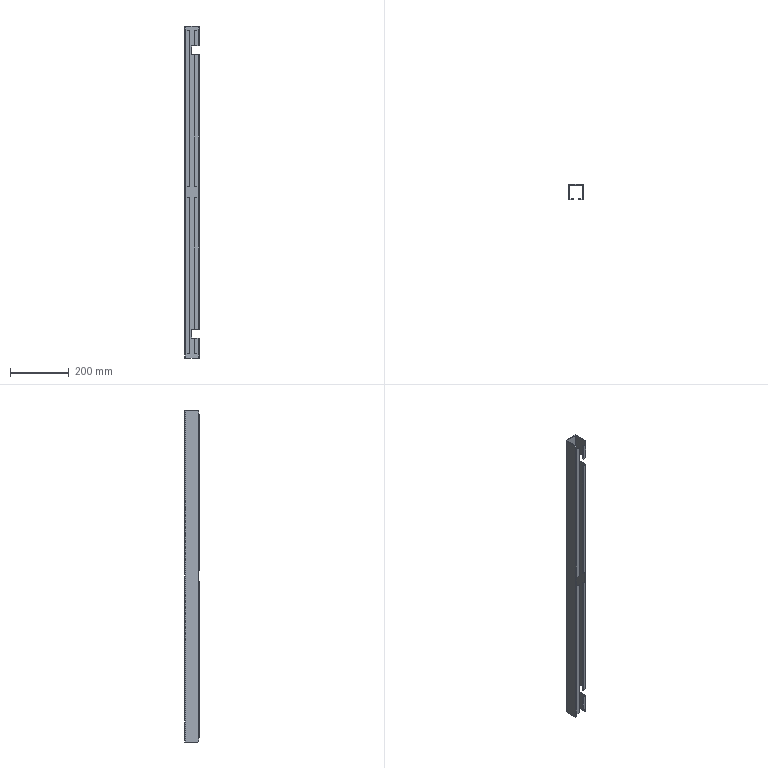Part | SolidWorks | features ICE 6, Chamfer 1, FlatPattern 1, SMBaseFlange 1, SheetMetal 1 | 1 solid | 102 faces | box 48 x 51 x 1130 mm | volume 366572 mm3 | plane 82 | cylinder 20 | commonest cylinder face diameters 2 x10 6 x10